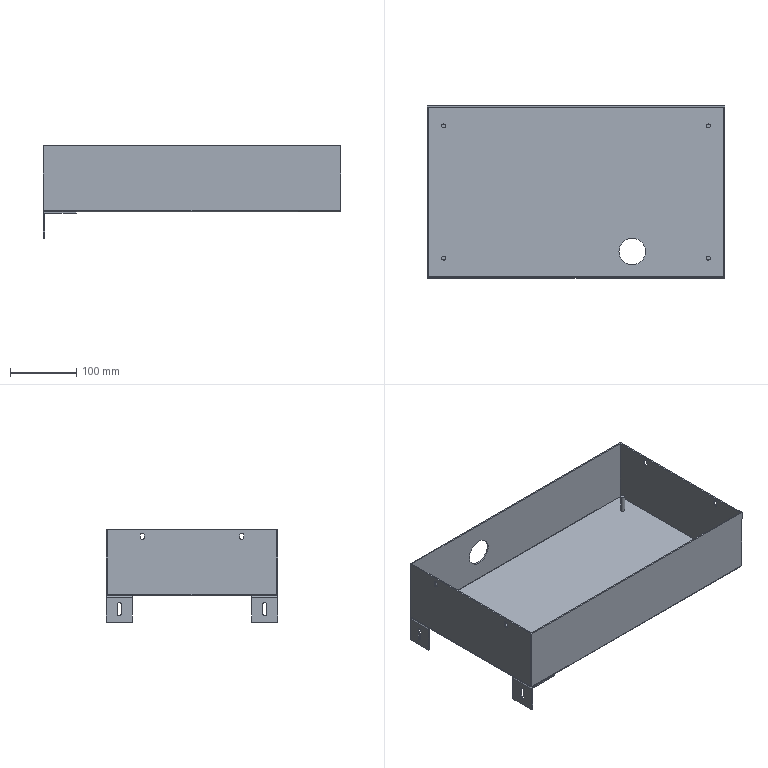Part | STEP file | CS-DS-004 | 3 solids | 122 faces | box 450 x 260 x 140 mm | volume 518743 mm3 | plane 70 | cylinder 44 | spline 8 | commonest cylinder face diameters 5.8 x12 6 x8 0.4 x6 4.4 x6 5.5 x6 40 x4